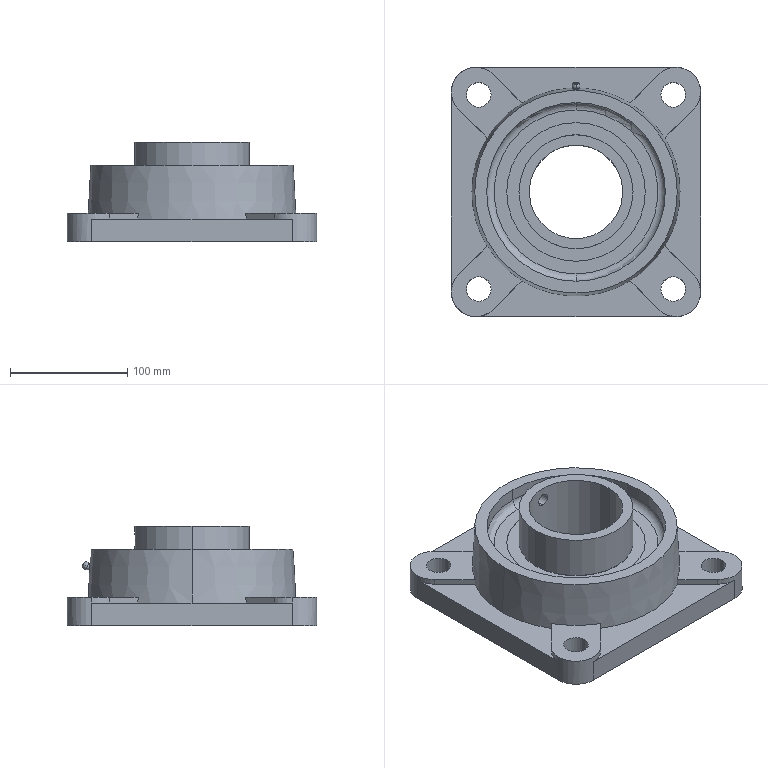Part | STEP file | GB/T7810-1995 square flange bearing UCFU216 | 1 solid | 118 faces | box 213 x 213 x 84.7 mm | volume 1127031 mm3 | cylinder 58 | plane 42 | sphere 10 | torus 6 | cone 2 | commonest cylinder face diameters 6 x14 42 x12 21 x8 97.4 x6 118.4 x6 152.6 x4